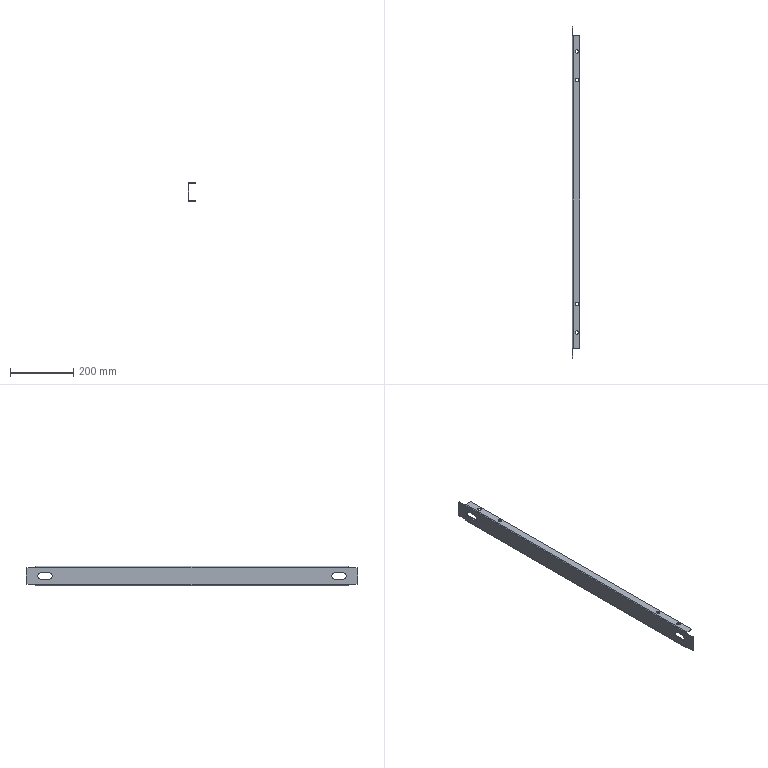Part | SolidWorks | features SMBaseFlange 2, Cut 1, Fillet 1, FlatPattern 1, ICE 1, SheetMetal 1 | 1 solid | 58 faces | box 25 x 1049 x 62 mm | volume 312113 mm3 | plane 30 | cylinder 28 | commonest cylinder face diameters 11 x16 6 x4 20 x4 0.4 x2 6.4 x2